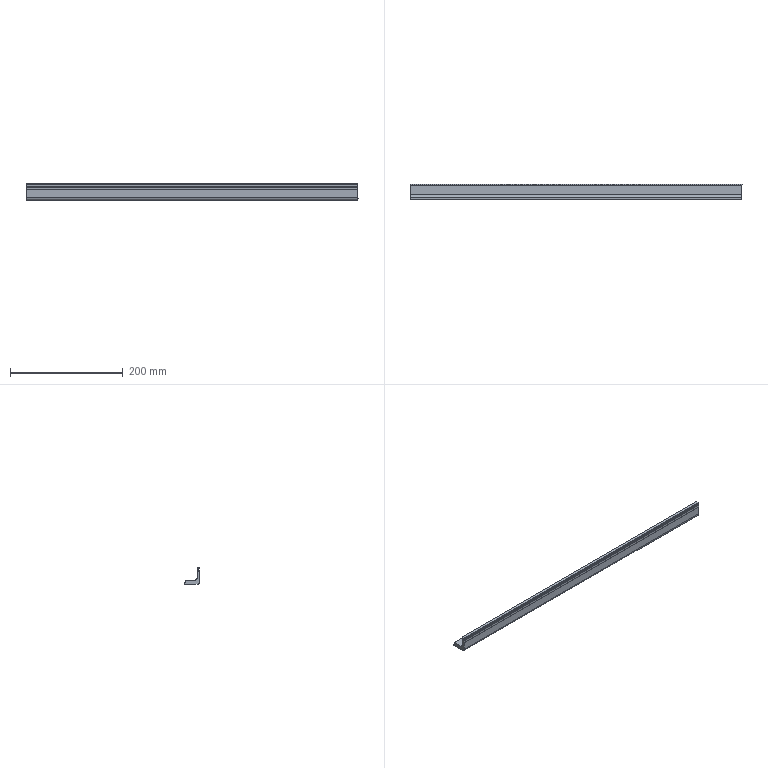Part | SolidWorks | features BaseBody 1 | 1 solid | 24 faces | box 590 x 28 x 29.5 mm | volume 170632 mm3 | plane 19 | cylinder 5 | commonest cylinder face diameters 0.6 x3 8 x1 10 x1
STEP:
#1=CARTESIAN_POINT('',(-288.521,1880.944,-97.5));
#2=VERTEX_POINT('',#1);
#3=CARTESIAN_POINT('',(-288.521,1881.244,-97.8));
#4=VERTEX_POINT('',#3);
#5=CARTESIAN_POINT('',(-288.521,1881.244,-97.5));
#6=DIRECTION('',(1.,0.,0.));
#7=DIRECTION('',(0.,0.,-1.));
#8=AXIS2_PLACEMENT_3D('',#5,#6,#7);
#9=CIRCLE('',#8,0.3);
#10=EDGE_CURVE('',#2,#4,#9,.T.);
#11=ORIENTED_EDGE('',*,*,#10,.T.);
#12=CARTESIAN_POINT('',(301.479,1881.244,-97.8));
#13=VERTEX_POINT('',#12);
#14=CARTESIAN_POINT('',(-288.521,1881.244,-97.8));
#15=DIRECTION('',(1.,0.,0.));
#16=VECTOR('',#15,1000.);
#17=LINE('',#14,#16);
#18=EDGE_CURVE('',#4,#13,#17,.T.);
#19=ORIENTED_EDGE('',*,*,#18,.T.);
#20=CARTESIAN_POINT('',(301.479,1880.944,-97.5));
#21=VERTEX_POINT('',#20);
#22=CARTESIAN_POINT('',(301.479,1881.244,-97.5));
#23=DIRECTION('',(1.,0.,0.));
#24=DIRECTION('',(0.,0.,-1.));
#25=AXIS2_PLACEMENT_3D('',#22,#23,#24);
#26=CIRCLE('',#25,0.3);
#27=EDGE_CURVE('',#21,#13,#26,.T.);
#28=ORIENTED_EDGE('',*,*,#27,.F.);
#29=CARTESIAN_POINT('',(-288.521,1880.944,-97.5));
#30=DIRECTION('',(-1.,0.,0.));
#31=VECTOR('',#30,1000.);
#32=LINE('',#29,#31);
#33=EDGE_CURVE('',#21,#2,#32,.T.);
#34=ORIENTED_EDGE('',*,*,#33,.T.);
#35=EDGE_LOOP('',(#11,#19,#28,#34));
#36=FACE_OUTER_BOUND('',#35,.T.);
#37=CARTESIAN_POINT('',(-288.521,1881.244,-97.5));
#38=DIRECTION('',(1.,0.,0.));
#39=DIRECTION('',(0.,0.,-1.));
#40=AXIS2_PLACEMENT_3D('',#37,#38,#39);
#41=CYLINDRICAL_SURFACE('',#40,0.3);
#42=ADVANCED_FACE('',(#36),#41,.T.);
#43=CARTESIAN_POINT('',(301.479,1884.544,-125.));
#44=VERTEX_POINT('',#43);
#45=CARTESIAN_POINT('',(-288.521,1884.544,-125.));
#46=VERTEX_POINT('',#45);
#47=CARTESIAN_POINT('',(-288.521,1884.544,-125.));
#48=DIRECTION('',(-1.,0.,0.));
#49=VECTOR('',#48,1000.);
#50=LINE('',#47,#49);
#51=EDGE_CURVE('',#44,#46,#50,.T.);
#52=ORIENTED_EDGE('',*,*,#51,.T.);
#53=CARTESIAN_POINT('',(-288.521,1907.544,-125.));
#54=VERTEX_POINT('',#53);
#55=CARTESIAN_POINT('',(-288.521,1907.544,-125.));
#56=DIRECTION('',(0.,1.,0.));
#57=VECTOR('',#56,1000.);
#58=LINE('',#55,#57);
#59=EDGE_CURVE('',#46,#54,#58,.T.);
#60=ORIENTED_EDGE('',*,*,#59,.T.);
#61=CARTESIAN_POINT('',(301.479,1907.544,-125.));
#62=VERTEX_POINT('',#61);
#63=CARTESIAN_POINT('',(-288.521,1907.544,-125.));
#64=DIRECTION('',(1.,0.,0.));
#65=VECTOR('',#64,1000.);
#66=LINE('',#63,#65);
#67=EDGE_CURVE('',#54,#62,#66,.T.);
#68=ORIENTED_EDGE('',*,*,#67,.T.);
#69=CARTESIAN_POINT('',(301.479,1907.544,-125.));
#70=DIRECTION('',(0.,-1.,0.));
#71=VECTOR('',#70,1000.);
#72=LINE('',#69,#71);
#73=EDGE_CURVE('',#62,#44,#72,.T.);
#74=ORIENTED_EDGE('',*,*,#73,.T.);
#75=EDGE_LOOP('',(#52,#60,#68,#74));
#76=FACE_OUTER_BOUND('',#75,.T.);
#77=CARTESIAN_POINT('',(-288.521,1907.544,-125.));
#78=DIRECTION('',(0.,0.,-1.));
#79=DIRECTION('',(0.,1.,0.));
#80=AXIS2_PLACEMENT_3D('',#77,#78,#79);
#81=PLANE('',#80);
#82=ADVANCED_FACE('',(#76),#81,.T.);
#83=CARTESIAN_POINT('',(-288.521,1907.544,-123.));
#84=VERTEX_POINT('',#83);
#85=CARTESIAN_POINT('',(-288.521,1907.544,-113.659));
#86=DIRECTION('',(0.,0.,1.));
#87=VECTOR('',#86,1000.);
#88=LINE('',#85,#87);
#89=EDGE_CURVE('',#54,#84,#88,.T.);
#90=ORIENTED_EDGE('',*,*,#89,.F.);
#91=ORIENTED_EDGE('',*,*,#59,.F.);
#92=CARTESIAN_POINT('',(-288.521,1879.544,-120.));
#93=VERTEX_POINT('',#92);
#94=CARTESIAN_POINT('',(-288.521,1884.544,-120.));
#95=DIRECTION('',(1.,0.,0.));
#96=DIRECTION('',(0.,0.,-1.));
#97=AXIS2_PLACEMENT_3D('',#94,#95,#96);
#98=CIRCLE('',#97,5.);
#99=EDGE_CURVE('',#93,#46,#98,.T.);
#100=ORIENTED_EDGE('',*,*,#99,.F.);
#101=CARTESIAN_POINT('',(-288.521,1879.544,-105.7));
#102=VERTEX_POINT('',#101);
#103=CARTESIAN_POINT('',(-288.521,1879.544,-113.659));
#104=DIRECTION('',(0.,0.,-1.));
#105=VECTOR('',#104,1000.);
#106=LINE('',#103,#105);
#107=EDGE_CURVE('',#102,#93,#106,.T.);
#108=ORIENTED_EDGE('',*,*,#107,.F.);
#109=CARTESIAN_POINT('',(-288.521,1879.744,-105.5));
#110=VERTEX_POINT('',#109);
#111=CARTESIAN_POINT('',(-288.521,1879.744,-105.5));
#112=DIRECTION('',(0.,-0.7071,-0.7071));
#113=VECTOR('',#112,1000.);
#114=LINE('',#111,#113);
#115=EDGE_CURVE('',#110,#102,#114,.T.);
#116=ORIENTED_EDGE('',*,*,#115,.F.);
#117=CARTESIAN_POINT('',(-288.521,1879.744,-101.5));
#118=VERTEX_POINT('',#117);
#119=CARTESIAN_POINT('',(-288.521,1879.744,-113.659));
#120=DIRECTION('',(0.,0.,-1.));
#121=VECTOR('',#120,1000.);
#122=LINE('',#119,#121);
#123=EDGE_CURVE('',#118,#110,#122,.T.);
#124=ORIENTED_EDGE('',*,*,#123,.F.);
#125=CARTESIAN_POINT('',(-288.521,1880.944,-101.5));
#126=VERTEX_POINT('',#125);
#127=CARTESIAN_POINT('',(-288.521,1888.924,-101.5));
#128=DIRECTION('',(0.,-1.,0.));
#129=VECTOR('',#128,1000.);
#130=LINE('',#127,#129);
#131=EDGE_CURVE('',#126,#118,#130,.T.);
#132=ORIENTED_EDGE('',*,*,#131,.F.);
#133=CARTESIAN_POINT('',(-288.521,1881.544,-101.5));
#134=VERTEX_POINT('',#133);
#135=CARTESIAN_POINT('',(-288.521,1881.244,-101.5));
#136=DIRECTION('',(1.,0.,0.));
#137=DIRECTION('',(0.,0.,-1.));
#138=AXIS2_PLACEMENT_3D('',#135,#136,#137);
#139=CIRCLE('',#138,0.3);
#140=EDGE_CURVE('',#134,#126,#139,.T.);
#141=ORIENTED_EDGE('',*,*,#140,.F.);
#142=CARTESIAN_POINT('',(-288.521,1882.744,-101.5));
#143=VERTEX_POINT('',#142);
#144=CARTESIAN_POINT('',(-288.521,1888.924,-101.5));
#145=DIRECTION('',(0.,-1.,0.));
#146=VECTOR('',#145,1000.);
#147=LINE('',#144,#146);
#148=EDGE_CURVE('',#143,#134,#147,.T.);
#149=ORIENTED_EDGE('',*,*,#148,.F.);
#150=CARTESIAN_POINT('',(-288.521,1882.744,-97.5));
#151=VERTEX_POINT('',#150);
#152=CARTESIAN_POINT('',(-288.521,1882.744,-113.659));
#153=DIRECTION('',(0.,0.,-1.));
#154=VECTOR('',#153,1000.);
#155=LINE('',#152,#154);
#156=EDGE_CURVE('',#151,#143,#155,.T.);
#157=ORIENTED_EDGE('',*,*,#156,.F.);
#158=CARTESIAN_POINT('',(-288.521,1881.544,-97.5));
#159=VERTEX_POINT('',#158);
#160=CARTESIAN_POINT('',(-288.521,1888.924,-97.5));
#161=DIRECTION('',(0.,1.,0.));
#162=VECTOR('',#161,1000.);
#163=LINE('',#160,#162);
#164=EDGE_CURVE('',#159,#151,#163,.T.);
#165=ORIENTED_EDGE('',*,*,#164,.F.);
#166=CARTESIAN_POINT('',(-288.521,1881.244,-97.5));
#167=DIRECTION('',(1.,0.,0.));
#168=DIRECTION('',(0.,0.,-1.));
#169=AXIS2_PLACEMENT_3D('',#166,#167,#168);
#170=CIRCLE('',#169,0.3);
#171=EDGE_CURVE('',#4,#159,#170,.T.);
#172=ORIENTED_EDGE('',*,*,#171,.F.);
#173=ORIENTED_EDGE('',*,*,#10,.F.);
#174=CARTESIAN_POINT('',(-288.521,1879.744,-97.5));
#175=VERTEX_POINT('',#174);
#176=CARTESIAN_POINT('',(-288.521,1888.924,-97.5));
#177=DIRECTION('',(0.,1.,0.));
#178=VECTOR('',#177,1000.);
#179=LINE('',#176,#178);
#180=EDGE_CURVE('',#175,#2,#179,.T.);
#181=ORIENTED_EDGE('',*,*,#180,.F.);
#182=CARTESIAN_POINT('',(-288.521,1879.744,-95.5));
#183=VERTEX_POINT('',#182);
#184=CARTESIAN_POINT('',(-288.521,1879.744,-113.659));
#185=DIRECTION('',(0.,0.,-1.));
#186=VECTOR('',#185,1000.);
#187=LINE('',#184,#186);
#188=EDGE_CURVE('',#183,#175,#187,.T.);
#189=ORIENTED_EDGE('',*,*,#188,.F.);
#190=CARTESIAN_POINT('',(-288.521,1884.544,-95.5));
#191=VERTEX_POINT('',#190);
#192=CARTESIAN_POINT('',(-288.521,1888.924,-95.5));
#193=DIRECTION('',(0.,-1.,0.));
#194=VECTOR('',#193,1000.);
#195=LINE('',#192,#194);
#196=EDGE_CURVE('',#191,#183,#195,.T.);
#197=ORIENTED_EDGE('',*,*,#196,.F.);
#198=CARTESIAN_POINT('',(-288.521,1884.544,-113.5));
#199=VERTEX_POINT('',#198);
#200=CARTESIAN_POINT('',(-288.521,1884.544,-113.659));
#201=DIRECTION('',(0.,0.,1.));
#202=VECTOR('',#201,1000.);
#203=LINE('',#200,#202);
#204=EDGE_CURVE('',#199,#191,#203,.T.);
#205=ORIENTED_EDGE('',*,*,#204,.F.);
#206=CARTESIAN_POINT('',(-288.521,1888.544,-117.5));
#207=VERTEX_POINT('',#206);
#208=CARTESIAN_POINT('',(-288.521,1888.544,-113.5));
#209=DIRECTION('',(-1.,0.,0.));
#210=DIRECTION('',(0.,0.,-1.));
#211=AXIS2_PLACEMENT_3D('',#208,#209,#210);
#212=CIRCLE('',#211,4.);
#213=EDGE_CURVE('',#207,#199,#212,.T.);
#214=ORIENTED_EDGE('',*,*,#213,.F.);
#215=CARTESIAN_POINT('',(-288.521,1904.544,-117.5));
#216=VERTEX_POINT('',#215);
#217=CARTESIAN_POINT('',(-288.521,1888.924,-117.5));
#218=DIRECTION('',(0.,-1.,0.));
#219=VECTOR('',#218,1000.);
#220=LINE('',#217,#219);
#221=EDGE_CURVE('',#216,#207,#220,.T.);
#222=ORIENTED_EDGE('',*,*,#221,.F.);
#223=CARTESIAN_POINT('',(-288.521,1904.544,-122.5));
#224=VERTEX_POINT('',#223);
#225=CARTESIAN_POINT('',(-288.521,1904.544,-113.659));
#226=DIRECTION('',(0.,0.,1.));
#227=VECTOR('',#226,1000.);
#228=LINE('',#225,#227);
#229=EDGE_CURVE('',#224,#216,#228,.T.);
#230=ORIENTED_EDGE('',*,*,#229,.F.);
#231=CARTESIAN_POINT('',(-288.521,1907.044,-122.5));
#232=VERTEX_POINT('',#231);
#233=CARTESIAN_POINT('',(-288.521,1888.924,-122.5));
#234=DIRECTION('',(0.,-1.,0.));
#235=VECTOR('',#234,1000.);
#236=LINE('',#233,#235);
#237=EDGE_CURVE('',#232,#224,#236,.T.);
#238=ORIENTED_EDGE('',*,*,#237,.F.);
#239=CARTESIAN_POINT('',(-288.521,1907.544,-123.));
#240=DIRECTION('',(0.,-0.7071,0.7071));
#241=VECTOR('',#240,1000.);
#242=LINE('',#239,#241);
#243=EDGE_CURVE('',#84,#232,#242,.T.);
#244=ORIENTED_EDGE('',*,*,#243,.F.);
#245=EDGE_LOOP('',(#90,#91,#100,#108,#116,#124,#132,#141,#149,#157,#165,#172,#173,#181,#189,#197,#205,#214,#222,#230,#238,#244));
#246=FACE_OUTER_BOUND('',#245,.T.);
#247=CARTESIAN_POINT('',(-288.521,1888.924,-113.659));
#248=DIRECTION('',(1.,0.,0.));
#249=DIRECTION('',(0.,0.,-1.));
#250=AXIS2_PLACEMENT_3D('',#247,#248,#249);
#251=PLANE('',#250);
#252=ADVANCED_FACE('',(#246),#251,.F.);
#253=CARTESIAN_POINT('',(301.479,1879.544,-120.));
#254=VERTEX_POINT('',#253);
#255=CARTESIAN_POINT('',(-288.521,1879.544,-120.));
#256=DIRECTION('',(-1.,0.,0.));
#257=VECTOR('',#256,1000.);
#258=LINE('',#255,#257);
#259=EDGE_CURVE('',#254,#93,#258,.T.);
#260=ORIENTED_EDGE('',*,*,#259,.T.);
#261=ORIENTED_EDGE('',*,*,#99,.T.);
#262=ORIENTED_EDGE('',*,*,#51,.F.);
#263=CARTESIAN_POINT('',(301.479,1884.544,-120.));
#264=DIRECTION('',(-1.,0.,0.));
#265=DIRECTION('',(0.,0.,-1.));
#266=AXIS2_PLACEMENT_3D('',#263,#264,#265);
#267=CIRCLE('',#266,5.);
#268=EDGE_CURVE('',#44,#254,#267,.T.);
#269=ORIENTED_EDGE('',*,*,#268,.T.);
#270=EDGE_LOOP('',(#260,#261,#262,#269));
#271=FACE_OUTER_BOUND('',#270,.T.);
#272=CARTESIAN_POINT('',(-288.521,1884.544,-120.));
#273=DIRECTION('',(1.,0.,0.));
#274=DIRECTION('',(0.,0.,-1.));
#275=AXIS2_PLACEMENT_3D('',#272,#273,#274);
#276=CYLINDRICAL_SURFACE('',#275,5.);
#277=ADVANCED_FACE('',(#271),#276,.T.);
#278=ORIENTED_EDGE('',*,*,#73,.F.);
#279=CARTESIAN_POINT('',(301.479,1907.544,-123.));
#280=VERTEX_POINT('',#279);
#281=CARTESIAN_POINT('',(301.479,1907.544,-113.659));
#282=DIRECTION('',(0.,0.,1.));
#283=VECTOR('',#282,1000.);
#284=LINE('',#281,#283);
#285=EDGE_CURVE('',#62,#280,#284,.T.);
#286=ORIENTED_EDGE('',*,*,#285,.T.);
#287=CARTESIAN_POINT('',(301.479,1907.044,-122.5));
#288=VERTEX_POINT('',#287);
#289=CARTESIAN_POINT('',(301.479,1907.544,-123.));
#290=DIRECTION('',(0.,-0.7071,0.7071));
#291=VECTOR('',#290,1000.);
#292=LINE('',#289,#291);
#293=EDGE_CURVE('',#280,#288,#292,.T.);
#294=ORIENTED_EDGE('',*,*,#293,.T.);
#295=CARTESIAN_POINT('',(301.479,1904.544,-122.5));
#296=VERTEX_POINT('',#295);
#297=CARTESIAN_POINT('',(301.479,1888.924,-122.5));
#298=DIRECTION('',(0.,-1.,0.));
#299=VECTOR('',#298,1000.);
#300=LINE('',#297,#299);
#301=EDGE_CURVE('',#288,#296,#300,.T.);
#302=ORIENTED_EDGE('',*,*,#301,.T.);
#303=CARTESIAN_POINT('',(301.479,1904.544,-117.5));
#304=VERTEX_POINT('',#303);
#305=CARTESIAN_POINT('',(301.479,1904.544,-113.659));
#306=DIRECTION('',(0.,0.,1.));
#307=VECTOR('',#306,1000.);
#308=LINE('',#305,#307);
#309=EDGE_CURVE('',#296,#304,#308,.T.);
#310=ORIENTED_EDGE('',*,*,#309,.T.);
#311=CARTESIAN_POINT('',(301.479,1888.544,-117.5));
#312=VERTEX_POINT('',#311);
#313=CARTESIAN_POINT('',(301.479,1888.924,-117.5));
#314=DIRECTION('',(0.,-1.,0.));
#315=VECTOR('',#314,1000.);
#316=LINE('',#313,#315);
#317=EDGE_CURVE('',#304,#312,#316,.T.);
#318=ORIENTED_EDGE('',*,*,#317,.T.);
#319=CARTESIAN_POINT('',(301.479,1884.544,-113.5));
#320=VERTEX_POINT('',#319);
#321=CARTESIAN_POINT('',(301.479,1888.544,-113.5));
#322=DIRECTION('',(-1.,0.,0.));
#323=DIRECTION('',(0.,0.,-1.));
#324=AXIS2_PLACEMENT_3D('',#321,#322,#323);
#325=CIRCLE('',#324,4.);
#326=EDGE_CURVE('',#312,#320,#325,.T.);
#327=ORIENTED_EDGE('',*,*,#326,.T.);
#328=CARTESIAN_POINT('',(301.479,1884.544,-95.5));
#329=VERTEX_POINT('',#328);
#330=CARTESIAN_POINT('',(301.479,1884.544,-113.659));
#331=DIRECTION('',(0.,0.,1.));
#332=VECTOR('',#331,1000.);
#333=LINE('',#330,#332);
#334=EDGE_CURVE('',#320,#329,#333,.T.);
#335=ORIENTED_EDGE('',*,*,#334,.T.);
#336=CARTESIAN_POINT('',(301.479,1879.744,-95.5));
#337=VERTEX_POINT('',#336);
#338=CARTESIAN_POINT('',(301.479,1888.924,-95.5));
#339=DIRECTION('',(0.,-1.,0.));
#340=VECTOR('',#339,1000.);
#341=LINE('',#338,#340);
#342=EDGE_CURVE('',#329,#337,#341,.T.);
#343=ORIENTED_EDGE('',*,*,#342,.T.);
#344=CARTESIAN_POINT('',(301.479,1879.744,-97.5));
#345=VERTEX_POINT('',#344);
#346=CARTESIAN_POINT('',(301.479,1879.744,-113.659));
#347=DIRECTION('',(0.,0.,-1.));
#348=VECTOR('',#347,1000.);
#349=LINE('',#346,#348);
#350=EDGE_CURVE('',#337,#345,#349,.T.);
#351=ORIENTED_EDGE('',*,*,#350,.T.);
#352=CARTESIAN_POINT('',(301.479,1888.924,-97.5));
#353=DIRECTION('',(0.,1.,0.));
#354=VECTOR('',#353,1000.);
#355=LINE('',#352,#354);
#356=EDGE_CURVE('',#345,#21,#355,.T.);
#357=ORIENTED_EDGE('',*,*,#356,.T.);
#358=ORIENTED_EDGE('',*,*,#27,.T.);
#359=CARTESIAN_POINT('',(301.479,1881.544,-97.5));
#360=VERTEX_POINT('',#359);
#361=CARTESIAN_POINT('',(301.479,1881.244,-97.5));
#362=DIRECTION('',(1.,0.,0.));
#363=DIRECTION('',(0.,0.,-1.));
#364=AXIS2_PLACEMENT_3D('',#361,#362,#363);
#365=CIRCLE('',#364,0.3);
#366=EDGE_CURVE('',#13,#360,#365,.T.);
#367=ORIENTED_EDGE('',*,*,#366,.T.);
#368=CARTESIAN_POINT('',(301.479,1882.744,-97.5));
#369=VERTEX_POINT('',#368);
#370=CARTESIAN_POINT('',(301.479,1888.924,-97.5));
#371=DIRECTION('',(0.,1.,0.));
#372=VECTOR('',#371,1000.);
#373=LINE('',#370,#372);
#374=EDGE_CURVE('',#360,#369,#373,.T.);
#375=ORIENTED_EDGE('',*,*,#374,.T.);
#376=CARTESIAN_POINT('',(301.479,1882.744,-101.5));
#377=VERTEX_POINT('',#376);
#378=CARTESIAN_POINT('',(301.479,1882.744,-113.659));
#379=DIRECTION('',(0.,0.,-1.));
#380=VECTOR('',#379,1000.);
#381=LINE('',#378,#380);
#382=EDGE_CURVE('',#369,#377,#381,.T.);
#383=ORIENTED_EDGE('',*,*,#382,.T.);
#384=CARTESIAN_POINT('',(301.479,1881.544,-101.5));
#385=VERTEX_POINT('',#384);
#386=CARTESIAN_POINT('',(301.479,1888.924,-101.5));
#387=DIRECTION('',(0.,-1.,0.));
#388=VECTOR('',#387,1000.);
#389=LINE('',#386,#388);
#390=EDGE_CURVE('',#377,#385,#389,.T.);
#391=ORIENTED_EDGE('',*,*,#390,.T.);
#392=CARTESIAN_POINT('',(301.479,1880.944,-101.5));
#393=VERTEX_POINT('',#392);
#394=CARTESIAN_POINT('',(301.479,1881.244,-101.5));
#395=DIRECTION('',(1.,0.,0.));
#396=DIRECTION('',(0.,0.,-1.));
#397=AXIS2_PLACEMENT_3D('',#394,#395,#396);
#398=CIRCLE('',#397,0.3);
#399=EDGE_CURVE('',#385,#393,#398,.T.);
#400=ORIENTED_EDGE('',*,*,#399,.T.);
#401=CARTESIAN_POINT('',(301.479,1879.744,-101.5));
#402=VERTEX_POINT('',#401);
#403=CARTESIAN_POINT('',(301.479,1888.924,-101.5));
#404=DIRECTION('',(0.,-1.,0.));
#405=VECTOR('',#404,1000.);
#406=LINE('',#403,#405);
#407=EDGE_CURVE('',#393,#402,#406,.T.);
#408=ORIENTED_EDGE('',*,*,#407,.T.);
#409=CARTESIAN_POINT('',(301.479,1879.744,-105.5));
#410=VERTEX_POINT('',#409);
#411=CARTESIAN_POINT('',(301.479,1879.744,-113.659));
#412=DIRECTION('',(0.,0.,-1.));
#413=VECTOR('',#412,1000.);
#414=LINE('',#411,#413);
#415=EDGE_CURVE('',#402,#410,#414,.T.);
#416=ORIENTED_EDGE('',*,*,#415,.T.);
#417=CARTESIAN_POINT('',(301.479,1879.544,-105.7));
#418=VERTEX_POINT('',#417);
#419=CARTESIAN_POINT('',(301.479,1879.744,-105.5));
#420=DIRECTION('',(0.,-0.7071,-0.7071));
#421=VECTOR('',#420,1000.);
#422=LINE('',#419,#421);
#423=EDGE_CURVE('',#410,#418,#422,.T.);
#424=ORIENTED_EDGE('',*,*,#423,.T.);
#425=CARTESIAN_POINT('',(301.479,1879.544,-113.659));
#426=DIRECTION('',(0.,0.,-1.));
#427=VECTOR('',#426,1000.);
#428=LINE('',#425,#427);
#429=EDGE_CURVE('',#418,#254,#428,.T.);
#430=ORIENTED_EDGE('',*,*,#429,.T.);
#431=ORIENTED_EDGE('',*,*,#268,.F.);
#432=EDGE_LOOP('',(#278,#286,#294,#302,#310,#318,#327,#335,#343,#351,#357,#358,#367,#375,#383,#391,#400,#408,#416,#424,#430,#431));
#433=FACE_OUTER_BOUND('',#432,.T.);
#434=CARTESIAN_POINT('',(301.479,1888.924,-113.659));
#435=DIRECTION('',(1.,0.,0.));
#436=DIRECTION('',(0.,0.,-1.));
#437=AXIS2_PLACEMENT_3D('',#434,#435,#436);
#438=PLANE('',#437);
#439=ADVANCED_FACE('',(#433),#438,.T.);
#440=ORIENTED_EDGE('',*,*,#67,.F.);
#441=ORIENTED_EDGE('',*,*,#89,.T.);
#442=CARTESIAN_POINT('',(-288.521,1907.544,-123.));
#443=DIRECTION('',(1.,0.,0.));
#444=VECTOR('',#443,1000.);
#445=LINE('',#442,#444);
#446=EDGE_CURVE('',#84,#280,#445,.T.);
#447=ORIENTED_EDGE('',*,*,#446,.T.);
#448=ORIENTED_EDGE('',*,*,#285,.F.);
#449=EDGE_LOOP('',(#440,#441,#447,#448));
#450=FACE_OUTER_BOUND('',#449,.T.);
#451=CARTESIAN_POINT('',(-288.521,1907.544,-123.));
#452=DIRECTION('',(0.,1.,0.));
#453=DIRECTION('',(0.,0.,1.));
#454=AXIS2_PLACEMENT_3D('',#451,#452,#453);
#455=PLANE('',#454);
#456=ADVANCED_FACE('',(#450),#455,.T.);
#457=ORIENTED_EDGE('',*,*,#446,.F.);
#458=ORIENTED_EDGE('',*,*,#243,.T.);
#459=CARTESIAN_POINT('',(-288.521,1907.044,-122.5));
#460=DIRECTION('',(1.,0.,0.));
#461=VECTOR('',#460,1000.);
#462=LINE('',#459,#461);
#463=EDGE_CURVE('',#232,#288,#462,.T.);
#464=ORIENTED_EDGE('',*,*,#463,.T.);
#465=ORIENTED_EDGE('',*,*,#293,.F.);
#466=EDGE_LOOP('',(#457,#458,#464,#465));
#467=FACE_OUTER_BOUND('',#466,.T.);
#468=CARTESIAN_POINT('',(-288.521,1907.044,-122.5));
#469=DIRECTION('',(0.,0.7071,0.7071));
#470=DIRECTION('',(0.,-0.7071,0.7071));
#471=AXIS2_PLACEMENT_3D('',#468,#469,#470);
#472=PLANE('',#471);
#473=ADVANCED_FACE('',(#467),#472,.T.);
#474=CARTESIAN_POINT('',(-288.521,1879.544,-105.7));
#475=DIRECTION('',(-1.,0.,0.));
#476=VECTOR('',#475,1000.);
#477=LINE('',#474,#476);
#478=EDGE_CURVE('',#418,#102,#477,.T.);
#479=ORIENTED_EDGE('',*,*,#478,.T.);
#480=ORIENTED_EDGE('',*,*,#107,.T.);
#481=ORIENTED_EDGE('',*,*,#259,.F.);
#482=ORIENTED_EDGE('',*,*,#429,.F.);
#483=EDGE_LOOP('',(#479,#480,#481,#482));
#484=FACE_OUTER_BOUND('',#483,.T.);
#485=CARTESIAN_POINT('',(-288.521,1879.544,-120.));
#486=DIRECTION('',(0.,-1.,0.));
#487=DIRECTION('',(0.,0.,-1.));
#488=AXIS2_PLACEMENT_3D('',#485,#486,#487);
#489=PLANE('',#488);
#490=ADVANCED_FACE('',(#484),#489,.T.);
#491=CARTESIAN_POINT('',(-288.521,1879.744,-105.5));
#492=DIRECTION('',(-1.,0.,0.));
#493=VECTOR('',#492,1000.);
#494=LINE('',#491,#493);
#495=EDGE_CURVE('',#410,#110,#494,.T.);
#496=ORIENTED_EDGE('',*,*,#495,.T.);
#497=ORIENTED_EDGE('',*,*,#115,.T.);
#498=ORIENTED_EDGE('',*,*,#478,.F.);
#499=ORIENTED_EDGE('',*,*,#423,.F.);
#500=EDGE_LOOP('',(#496,#497,#498,#499));
#501=FACE_OUTER_BOUND('',#500,.T.);
#502=CARTESIAN_POINT('',(-288.521,1879.544,-105.7));
#503=DIRECTION('',(0.,-0.7071,0.7071));
#504=DIRECTION('',(0.,-0.7071,-0.7071));
#505=AXIS2_PLACEMENT_3D('',#502,#503,#504);
#506=PLANE('',#505);
#507=ADVANCED_FACE('',(#501),#506,.T.);
#508=CARTESIAN_POINT('',(-288.521,1879.744,-101.5));
#509=DIRECTION('',(-1.,0.,0.));
#510=VECTOR('',#509,1000.);
#511=LINE('',#508,#510);
#512=EDGE_CURVE('',#402,#118,#511,.T.);
#513=ORIENTED_EDGE('',*,*,#512,.T.);
#514=ORIENTED_EDGE('',*,*,#123,.T.);
#515=ORIENTED_EDGE('',*,*,#495,.F.);
#516=ORIENTED_EDGE('',*,*,#415,.F.);
#517=EDGE_LOOP('',(#513,#514,#515,#516));
#518=FACE_OUTER_BOUND('',#517,.T.);
#519=CARTESIAN_POINT('',(-288.521,1879.744,-105.5));
#520=DIRECTION('',(0.,-1.,0.));
#521=DIRECTION('',(0.,0.,-1.));
#522=AXIS2_PLACEMENT_3D('',#519,#520,#521);
#523=PLANE('',#522);
#524=ADVANCED_FACE('',(#518),#523,.T.);
#525=CARTESIAN_POINT('',(-288.521,1880.944,-101.5));
#526=DIRECTION('',(-1.,0.,0.));
#527=VECTOR('',#526,1000.);
#528=LINE('',#525,#527);
#529=EDGE_CURVE('',#393,#126,#528,.T.);
#530=ORIENTED_EDGE('',*,*,#529,.T.);
#531=ORIENTED_EDGE('',*,*,#131,.T.);
#532=ORIENTED_EDGE('',*,*,#512,.F.);
#533=ORIENTED_EDGE('',*,*,#407,.F.);
#534=EDGE_LOOP('',(#530,#531,#532,#533));
#535=FACE_OUTER_BOUND('',#534,.T.);
#536=CARTESIAN_POINT('',(-288.521,1879.744,-101.5));
#537=DIRECTION('',(0.,0.,1.));
#538=DIRECTION('',(1.,0.,0.));
#539=AXIS2_PLACEMENT_3D('',#536,#537,#538);
#540=PLANE('',#539);
#541=ADVANCED_FACE('',(#535),#540,.T.);
#542=CARTESIAN_POINT('',(-288.521,1881.544,-101.5));
#543=DIRECTION('',(-1.,0.,0.));
#544=VECTOR('',#543,1000.);
#545=LINE('',#542,#544);
#546=EDGE_CURVE('',#385,#134,#545,.T.);
#547=ORIENTED_EDGE('',*,*,#546,.T.);
#548=ORIENTED_EDGE('',*,*,#140,.T.);
#549=ORIENTED_EDGE('',*,*,#529,.F.);
#550=ORIENTED_EDGE('',*,*,#399,.F.);
#551=EDGE_LOOP('',(#547,#548,#549,#550));
#552=FACE_OUTER_BOUND('',#551,.T.);
#553=CARTESIAN_POINT('',(-288.521,1881.244,-101.5));
#554=DIRECTION('',(1.,0.,0.));
#555=DIRECTION('',(0.,0.,-1.));
#556=AXIS2_PLACEMENT_3D('',#553,#554,#555);
#557=CYLINDRICAL_SURFACE('',#556,0.3);
#558=ADVANCED_FACE('',(#552),#557,.T.);
#559=CARTESIAN_POINT('',(-288.521,1882.744,-101.5));
#560=DIRECTION('',(-1.,0.,0.));
#561=VECTOR('',#560,1000.);
#562=LINE('',#559,#561);
#563=EDGE_CURVE('',#377,#143,#562,.T.);
#564=ORIENTED_EDGE('',*,*,#563,.T.);
#565=ORIENTED_EDGE('',*,*,#148,.T.);
#566=ORIENTED_EDGE('',*,*,#546,.F.);
#567=ORIENTED_EDGE('',*,*,#390,.F.);
#568=EDGE_LOOP('',(#564,#565,#566,#567));
#569=FACE_OUTER_BOUND('',#568,.T.);
#570=CARTESIAN_POINT('',(-288.521,1881.544,-101.5));
#571=DIRECTION('',(0.,0.,1.));
#572=DIRECTION('',(1.,0.,0.));
#573=AXIS2_PLACEMENT_3D('',#570,#571,#572);
#574=PLANE('',#573);
#575=ADVANCED_FACE('',(#569),#574,.T.);
#576=CARTESIAN_POINT('',(-288.521,1882.744,-97.5));
#577=DIRECTION('',(-1.,0.,0.));
#578=VECTOR('',#577,1000.);
#579=LINE('',#576,#578);
#580=EDGE_CURVE('',#369,#151,#579,.T.);
#581=ORIENTED_EDGE('',*,*,#580,.T.);
#582=ORIENTED_EDGE('',*,*,#156,.T.);
#583=ORIENTED_EDGE('',*,*,#563,.F.);
#584=ORIENTED_EDGE('',*,*,#382,.F.);
#585=EDGE_LOOP('',(#581,#582,#583,#584));
#586=FACE_OUTER_BOUND('',#585,.T.);
#587=CARTESIAN_POINT('',(-288.521,1882.744,-101.5));
#588=DIRECTION('',(0.,-1.,0.));
#589=DIRECTION('',(0.,0.,-1.));
#590=AXIS2_PLACEMENT_3D('',#587,#588,#589);
#591=PLANE('',#590);
#592=ADVANCED_FACE('',(#586),#591,.T.);
#593=CARTESIAN_POINT('',(-288.521,1881.544,-97.5));
#594=DIRECTION('',(-1.,0.,0.));
#595=VECTOR('',#594,1000.);
#596=LINE('',#593,#595);
#597=EDGE_CURVE('',#360,#159,#596,.T.);
#598=ORIENTED_EDGE('',*,*,#597,.T.);
#599=ORIENTED_EDGE('',*,*,#164,.T.);
#600=ORIENTED_EDGE('',*,*,#580,.F.);
#601=ORIENTED_EDGE('',*,*,#374,.F.);
#602=EDGE_LOOP('',(#598,#599,#600,#601));
#603=FACE_OUTER_BOUND('',#602,.T.);
#604=CARTESIAN_POINT('',(-288.521,1882.744,-97.5));
#605=DIRECTION('',(0.,0.,-1.));
#606=DIRECTION('',(-1.,0.,0.));
#607=AXIS2_PLACEMENT_3D('',#604,#605,#606);
#608=PLANE('',#607);
#609=ADVANCED_FACE('',(#603),#608,.T.);
#610=ORIENTED_EDGE('',*,*,#18,.F.);
#611=ORIENTED_EDGE('',*,*,#171,.T.);
#612=ORIENTED_EDGE('',*,*,#597,.F.);
#613=ORIENTED_EDGE('',*,*,#366,.F.);
#614=EDGE_LOOP('',(#610,#611,#612,#613));
#615=FACE_OUTER_BOUND('',#614,.T.);
#616=CARTESIAN_POINT('',(-288.521,1881.244,-97.5));
#617=DIRECTION('',(1.,0.,0.));
#618=DIRECTION('',(0.,0.,-1.));
#619=AXIS2_PLACEMENT_3D('',#616,#617,#618);
#620=CYLINDRICAL_SURFACE('',#619,0.3);
#621=ADVANCED_FACE('',(#615),#620,.T.);
#622=CARTESIAN_POINT('',(-288.521,1879.744,-97.5));
#623=DIRECTION('',(-1.,0.,0.));
#624=VECTOR('',#623,1000.);
#625=LINE('',#622,#624);
#626=EDGE_CURVE('',#345,#175,#625,.T.);
#627=ORIENTED_EDGE('',*,*,#626,.T.);
#628=ORIENTED_EDGE('',*,*,#180,.T.);
#629=ORIENTED_EDGE('',*,*,#33,.F.);
#630=ORIENTED_EDGE('',*,*,#356,.F.);
#631=EDGE_LOOP('',(#627,#628,#629,#630));
#632=FACE_OUTER_BOUND('',#631,.T.);
#633=CARTESIAN_POINT('',(-288.521,1880.944,-97.5));
#634=DIRECTION('',(0.,0.,-1.));
#635=DIRECTION('',(-1.,0.,0.));
#636=AXIS2_PLACEMENT_3D('',#633,#634,#635);
#637=PLANE('',#636);
#638=ADVANCED_FACE('',(#632),#637,.T.);
#639=CARTESIAN_POINT('',(-288.521,1879.744,-95.5));
#640=DIRECTION('',(-1.,0.,0.));
#641=VECTOR('',#640,1000.);
#642=LINE('',#639,#641);
#643=EDGE_CURVE('',#337,#183,#642,.T.);
#644=ORIENTED_EDGE('',*,*,#643,.T.);
#645=ORIENTED_EDGE('',*,*,#188,.T.);
#646=ORIENTED_EDGE('',*,*,#626,.F.);
#647=ORIENTED_EDGE('',*,*,#350,.F.);
#648=EDGE_LOOP('',(#644,#645,#646,#647));
#649=FACE_OUTER_BOUND('',#648,.T.);
#650=CARTESIAN_POINT('',(-288.521,1879.744,-97.5));
#651=DIRECTION('',(0.,-1.,0.));
#652=DIRECTION('',(0.,0.,-1.));
#653=AXIS2_PLACEMENT_3D('',#650,#651,#652);
#654=PLANE('',#653);
#655=ADVANCED_FACE('',(#649),#654,.T.);
#656=CARTESIAN_POINT('',(-288.521,1884.544,-95.5));
#657=DIRECTION('',(-1.,0.,0.));
#658=VECTOR('',#657,1000.);
#659=LINE('',#656,#658);
#660=EDGE_CURVE('',#329,#191,#659,.T.);
#661=ORIENTED_EDGE('',*,*,#660,.T.);
#662=ORIENTED_EDGE('',*,*,#196,.T.);
#663=ORIENTED_EDGE('',*,*,#643,.F.);
#664=ORIENTED_EDGE('',*,*,#342,.F.);
#665=EDGE_LOOP('',(#661,#662,#663,#664));
#666=FACE_OUTER_BOUND('',#665,.T.);
#667=CARTESIAN_POINT('',(-288.521,1879.744,-95.5));
#668=DIRECTION('',(0.,0.,1.));
#669=DIRECTION('',(1.,0.,0.));
#670=AXIS2_PLACEMENT_3D('',#667,#668,#669);
#671=PLANE('',#670);
#672=ADVANCED_FACE('',(#666),#671,.T.);
#673=CARTESIAN_POINT('',(-288.521,1884.544,-113.5));
#674=DIRECTION('',(-1.,0.,0.));
#675=VECTOR('',#674,1000.);
#676=LINE('',#673,#675);
#677=EDGE_CURVE('',#320,#199,#676,.T.);
#678=ORIENTED_EDGE('',*,*,#677,.T.);
#679=ORIENTED_EDGE('',*,*,#204,.T.);
#680=ORIENTED_EDGE('',*,*,#660,.F.);
#681=ORIENTED_EDGE('',*,*,#334,.F.);
#682=EDGE_LOOP('',(#678,#679,#680,#681));
#683=FACE_OUTER_BOUND('',#682,.T.);
#684=CARTESIAN_POINT('',(-288.521,1884.544,-95.5));
#685=DIRECTION('',(0.,1.,0.));
#686=DIRECTION('',(0.,0.,1.));
#687=AXIS2_PLACEMENT_3D('',#684,#685,#686);
#688=PLANE('',#687);
#689=ADVANCED_FACE('',(#683),#688,.T.);
#690=ORIENTED_EDGE('',*,*,#677,.F.);
#691=ORIENTED_EDGE('',*,*,#326,.F.);
#692=CARTESIAN_POINT('',(-288.521,1888.544,-117.5));
#693=DIRECTION('',(1.,0.,0.));
#694=VECTOR('',#693,1000.);
#695=LINE('',#692,#694);
#696=EDGE_CURVE('',#207,#312,#695,.T.);
#697=ORIENTED_EDGE('',*,*,#696,.F.);
#698=ORIENTED_EDGE('',*,*,#213,.T.);
#699=EDGE_LOOP('',(#690,#691,#697,#698));
#700=FACE_OUTER_BOUND('',#699,.T.);
#701=CARTESIAN_POINT('',(-288.521,1888.544,-113.5));
#702=DIRECTION('',(1.,0.,0.));
#703=DIRECTION('',(0.,0.,-1.));
#704=AXIS2_PLACEMENT_3D('',#701,#702,#703);
#705=CYLINDRICAL_SURFACE('',#704,4.);
#706=ADVANCED_FACE('',(#700),#705,.F.);
#707=CARTESIAN_POINT('',(-288.521,1904.544,-117.5));
#708=DIRECTION('',(-1.,0.,0.));
#709=VECTOR('',#708,1000.);
#710=LINE('',#707,#709);
#711=EDGE_CURVE('',#304,#216,#710,.T.);
#712=ORIENTED_EDGE('',*,*,#711,.T.);
#713=ORIENTED_EDGE('',*,*,#221,.T.);
#714=ORIENTED_EDGE('',*,*,#696,.T.);
#715=ORIENTED_EDGE('',*,*,#317,.F.);
#716=EDGE_LOOP('',(#712,#713,#714,#715));
#717=FACE_OUTER_BOUND('',#716,.T.);
#718=CARTESIAN_POINT('',(-288.521,1888.544,-117.5));
#719=DIRECTION('',(0.,0.,1.));
#720=DIRECTION('',(0.,-1.,0.));
#721=AXIS2_PLACEMENT_3D('',#718,#719,#720);
#722=PLANE('',#721);
#723=ADVANCED_FACE('',(#717),#722,.T.);
#724=CARTESIAN_POINT('',(-288.521,1904.544,-122.5));
#725=DIRECTION('',(-1.,0.,0.));
#726=VECTOR('',#725,1000.);
#727=LINE('',#724,#726);
#728=EDGE_CURVE('',#296,#224,#727,.T.);
#729=ORIENTED_EDGE('',*,*,#728,.T.);
#730=ORIENTED_EDGE('',*,*,#229,.T.);
#731=ORIENTED_EDGE('',*,*,#711,.F.);
#732=ORIENTED_EDGE('',*,*,#309,.F.);
#733=EDGE_LOOP('',(#729,#730,#731,#732));
#734=FACE_OUTER_BOUND('',#733,.T.);
#735=CARTESIAN_POINT('',(-288.521,1904.544,-117.5));
#736=DIRECTION('',(0.,1.,0.));
#737=DIRECTION('',(0.,0.,1.));
#738=AXIS2_PLACEMENT_3D('',#735,#736,#737);
#739=PLANE('',#738);
#740=ADVANCED_FACE('',(#734),#739,.T.);
#741=ORIENTED_EDGE('',*,*,#463,.F.);
#742=ORIENTED_EDGE('',*,*,#237,.T.);
#743=ORIENTED_EDGE('',*,*,#728,.F.);
#744=ORIENTED_EDGE('',*,*,#301,.F.);
#745=EDGE_LOOP('',(#741,#742,#743,#744));
#746=FACE_OUTER_BOUND('',#745,.T.);
#747=CARTESIAN_POINT('',(-288.521,1904.544,-122.5));
#748=DIRECTION('',(0.,0.,1.));
#749=DIRECTION('',(0.,-1.,0.));
#750=AXIS2_PLACEMENT_3D('',#747,#748,#749);
#751=PLANE('',#750);
#752=ADVANCED_FACE('',(#746),#751,.T.);
#753=CLOSED_SHELL('',(#42,#82,#252,#277,#439,#456,#473,#490,#507,#524,#541,#558,#575,#592,#609,#621,#638,#655,#672,#689,#706,#723,#740,#752));
#754=MANIFOLD_SOLID_BREP('',#753);
#755=CARTESIAN_POINT('',(0.,0.,0.));
#756=DIRECTION('',(0.,0.,1.));
#757=DIRECTION('',(1.,0.,0.));
#758=AXIS2_PLACEMENT_3D('',#755,#756,#757);
#759=(LENGTH_UNIT()NAMED_UNIT(*)SI_UNIT(.MILLI.,.METRE.));
#760=UNCERTAINTY_MEASURE_WITH_UNIT(LENGTH_MEASURE(0.00001),#759,'','');
#761=(NAMED_UNIT(*)PLANE_ANGLE_UNIT()SI_UNIT($,.RADIAN.));
#762=(NAMED_UNIT(*)SI_UNIT($,.STERADIAN.)SOLID_ANGLE_UNIT());
#763=(GEOMETRIC_REPRESENTATION_CONTEXT(3)GLOBAL_UNCERTAINTY_ASSIGNED_CONTEXT((#760))GLOBAL_UNIT_ASSIGNED_CONTEXT((#759,#761,#762))REPRESENTATION_CONTEXT('',''));
#764=ADVANCED_BREP_SHAPE_REPRESENTATION('',(#754,#758),#763);